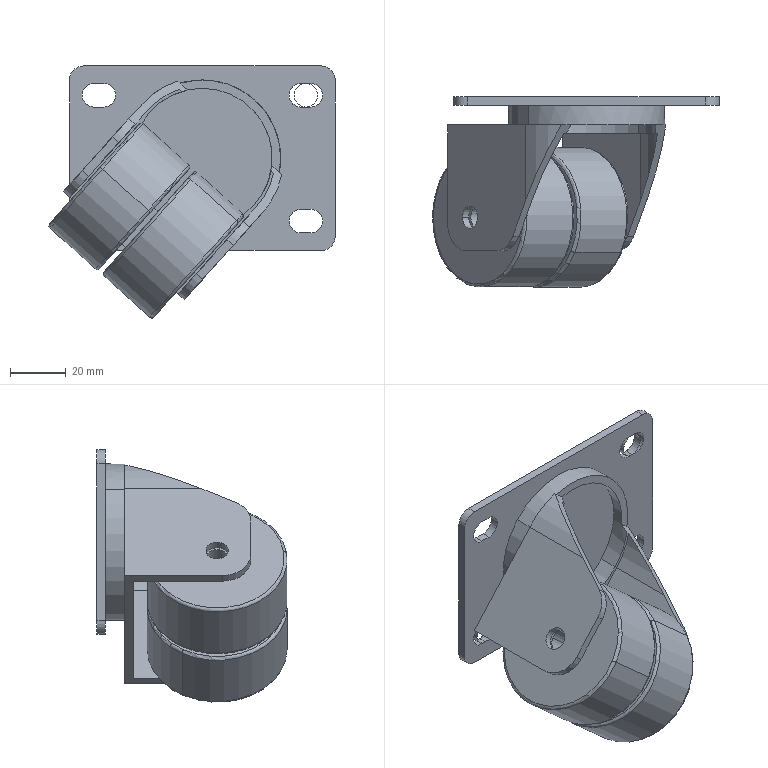Part | SolidWorks | 3 solids | 85 faces | box 102.422 x 68 x 90.224 mm | volume 133824 mm3 | cylinder 44 | plane 33 | torus 8 | commonest cylinder face diameters 8.4 x12 8 x8 50 x6 10 x4 20 x4 25 x4